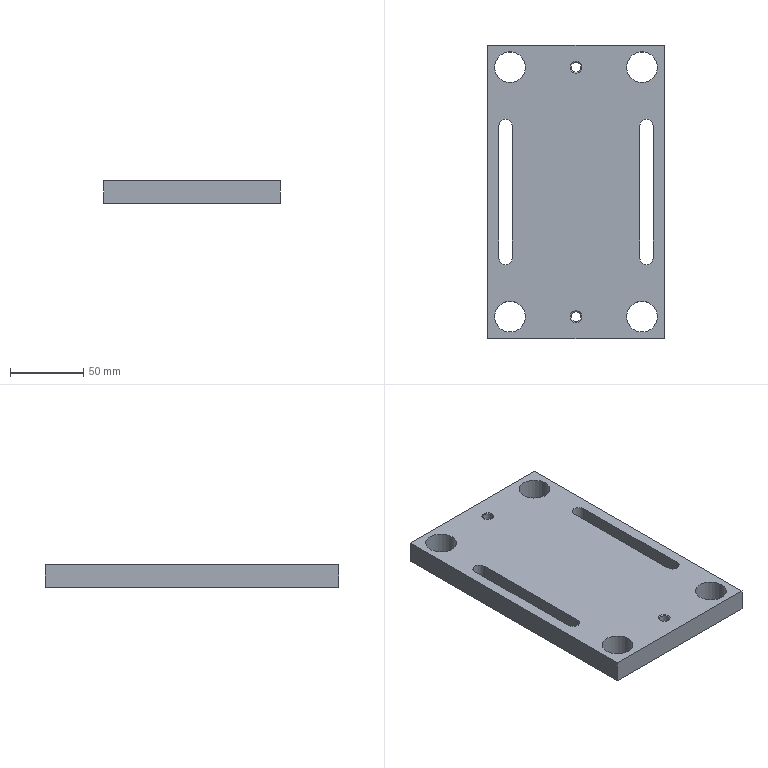Part | STEP file | 冲床-300配套压波_id874_x_t | 1 solid | 72 faces | box 120 x 200 x 15 mm | volume 311095 mm3 | cone 36 | cylinder 26 | plane 10 | commonest cylinder face diameters 2.5 x16 9 x4 21 x4 6.8 x2